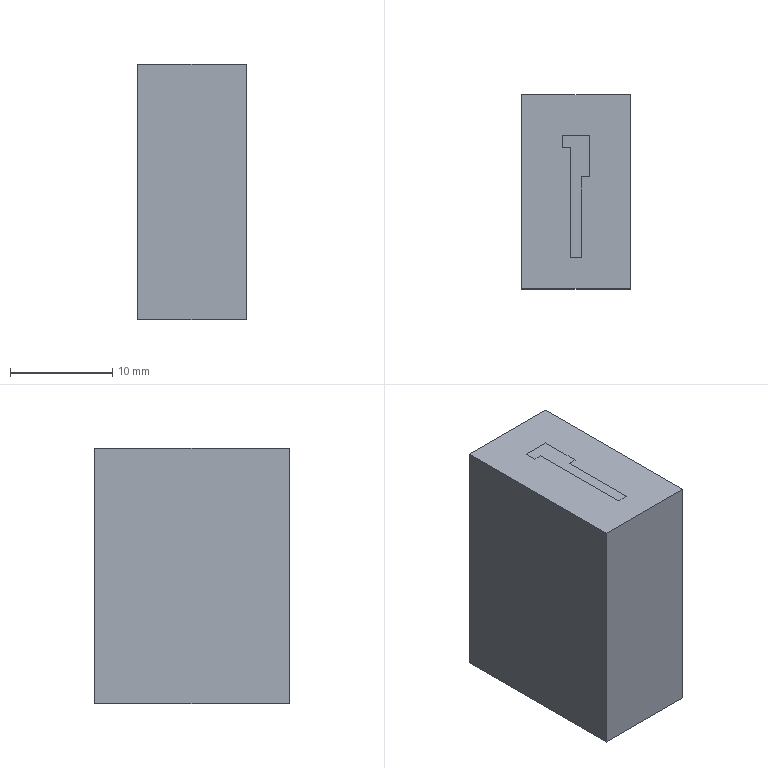Part | NX | features BREP 2 | 2 solids | 29 faces | box 10.58 x 19 x 25 mm | volume 8888 mm3 | plane 29
STEP:
#1=CARTESIAN_POINT('',(-5.29,-9.052,-25.6));
#2=VERTEX_POINT('',#1);
#3=CARTESIAN_POINT('',(-5.29,9.948,-25.6));
#4=VERTEX_POINT('',#3);
#5=CARTESIAN_POINT('',(-5.29,-9.052,-25.6));
#6=DIRECTION('',(0.,1.,0.));
#7=VECTOR('',#6,1000.);
#8=LINE('',#5,#7);
#9=EDGE_CURVE('',#2,#4,#8,.T.);
#10=ORIENTED_EDGE('',*,*,#9,.T.);
#11=CARTESIAN_POINT('',(5.29,9.948,-25.6));
#12=VERTEX_POINT('',#11);
#13=CARTESIAN_POINT('',(-5.29,9.948,-25.6));
#14=DIRECTION('',(1.,0.,0.));
#15=VECTOR('',#14,1000.);
#16=LINE('',#13,#15);
#17=EDGE_CURVE('',#4,#12,#16,.T.);
#18=ORIENTED_EDGE('',*,*,#17,.T.);
#19=CARTESIAN_POINT('',(5.29,-9.052,-25.6));
#20=VERTEX_POINT('',#19);
#21=CARTESIAN_POINT('',(5.29,9.948,-25.6));
#22=DIRECTION('',(0.,-1.,0.));
#23=VECTOR('',#22,1000.);
#24=LINE('',#21,#23);
#25=EDGE_CURVE('',#12,#20,#24,.T.);
#26=ORIENTED_EDGE('',*,*,#25,.T.);
#27=CARTESIAN_POINT('',(5.29,-9.052,-25.6));
#28=DIRECTION('',(-1.,0.,0.));
#29=VECTOR('',#28,1000.);
#30=LINE('',#27,#29);
#31=EDGE_CURVE('',#20,#2,#30,.T.);
#32=ORIENTED_EDGE('',*,*,#31,.T.);
#33=EDGE_LOOP('',(#10,#18,#26,#32));
#34=FACE_BOUND('',#33,.T.);
#35=CARTESIAN_POINT('',(-1.54,3.805,-25.6));
#36=VERTEX_POINT('',#35);
#37=CARTESIAN_POINT('',(-1.54,-6.998,-25.6));
#38=VERTEX_POINT('',#37);
#39=CARTESIAN_POINT('',(-1.54,-2.355,-25.6));
#40=DIRECTION('',(0.,-1.,0.));
#41=VECTOR('',#40,1000.);
#42=LINE('',#39,#41);
#43=EDGE_CURVE('',#36,#38,#42,.T.);
#44=ORIENTED_EDGE('',*,*,#43,.T.);
#45=CARTESIAN_POINT('',(1.54,-6.998,-25.6));
#46=VERTEX_POINT('',#45);
#47=CARTESIAN_POINT('',(-7.04,-6.998,-25.6));
#48=DIRECTION('',(1.,0.,0.));
#49=VECTOR('',#48,1000.);
#50=LINE('',#47,#49);
#51=EDGE_CURVE('',#38,#46,#50,.T.);
#52=ORIENTED_EDGE('',*,*,#51,.T.);
#53=CARTESIAN_POINT('',(1.54,0.9052,-25.6));
#54=VERTEX_POINT('',#53);
#55=CARTESIAN_POINT('',(1.54,-5.255,-25.6));
#56=DIRECTION('',(0.,1.,0.));
#57=VECTOR('',#56,1000.);
#58=LINE('',#55,#57);
#59=EDGE_CURVE('',#46,#54,#58,.T.);
#60=ORIENTED_EDGE('',*,*,#59,.T.);
#61=CARTESIAN_POINT('',(2.34,0.9052,-25.6));
#62=VERTEX_POINT('',#61);
#63=CARTESIAN_POINT('',(1.29,0.9052,-25.6));
#64=DIRECTION('',(1.,0.,0.));
#65=VECTOR('',#64,1000.);
#66=LINE('',#63,#65);
#67=EDGE_CURVE('',#54,#62,#66,.T.);
#68=ORIENTED_EDGE('',*,*,#67,.T.);
#69=CARTESIAN_POINT('',(2.34,6.998,-25.6));
#70=VERTEX_POINT('',#69);
#71=CARTESIAN_POINT('',(2.34,5.948,-25.6));
#72=DIRECTION('',(0.,1.,0.));
#73=VECTOR('',#72,1000.);
#74=LINE('',#71,#73);
#75=EDGE_CURVE('',#62,#70,#74,.T.);
#76=ORIENTED_EDGE('',*,*,#75,.T.);
#77=CARTESIAN_POINT('',(-2.34,6.998,-25.6));
#78=VERTEX_POINT('',#77);
#79=CARTESIAN_POINT('',(-7.04,6.998,-25.6));
#80=DIRECTION('',(-1.,0.,0.));
#81=VECTOR('',#80,1000.);
#82=LINE('',#79,#81);
#83=EDGE_CURVE('',#70,#78,#82,.T.);
#84=ORIENTED_EDGE('',*,*,#83,.T.);
#85=CARTESIAN_POINT('',(-2.34,3.805,-25.6));
#86=VERTEX_POINT('',#85);
#87=CARTESIAN_POINT('',(-2.34,4.855,-25.6));
#88=DIRECTION('',(0.,-1.,0.));
#89=VECTOR('',#88,1000.);
#90=LINE('',#87,#89);
#91=EDGE_CURVE('',#78,#86,#90,.T.);
#92=ORIENTED_EDGE('',*,*,#91,.T.);
#93=CARTESIAN_POINT('',(-0.4899,3.805,-25.6));
#94=DIRECTION('',(1.,0.,0.));
#95=VECTOR('',#94,1000.);
#96=LINE('',#93,#95);
#97=EDGE_CURVE('',#86,#36,#96,.T.);
#98=ORIENTED_EDGE('',*,*,#97,.T.);
#99=EDGE_LOOP('',(#44,#52,#60,#68,#76,#84,#92,#98));
#100=FACE_BOUND('',#99,.T.);
#101=CARTESIAN_POINT('',(0.,0.,-25.6));
#102=DIRECTION('',(0.,0.,-1.));
#103=DIRECTION('',(1.,0.,0.));
#104=AXIS2_PLACEMENT_3D('',#101,#102,#103);
#105=PLANE('',#104);
#106=ADVANCED_FACE('',(#34,#100),#105,.T.);
#107=CARTESIAN_POINT('',(-5.29,-9.052,-0.6));
#108=VERTEX_POINT('',#107);
#109=CARTESIAN_POINT('',(-5.29,9.948,-0.6));
#110=VERTEX_POINT('',#109);
#111=CARTESIAN_POINT('',(-5.29,-9.052,-0.6));
#112=DIRECTION('',(0.,1.,0.));
#113=VECTOR('',#112,1000.);
#114=LINE('',#111,#113);
#115=EDGE_CURVE('',#108,#110,#114,.T.);
#116=ORIENTED_EDGE('',*,*,#115,.F.);
#117=CARTESIAN_POINT('',(5.29,-9.052,-0.6));
#118=VERTEX_POINT('',#117);
#119=CARTESIAN_POINT('',(5.29,-9.052,-0.6));
#120=DIRECTION('',(-1.,0.,0.));
#121=VECTOR('',#120,1000.);
#122=LINE('',#119,#121);
#123=EDGE_CURVE('',#118,#108,#122,.T.);
#124=ORIENTED_EDGE('',*,*,#123,.F.);
#125=CARTESIAN_POINT('',(5.29,9.948,-0.6));
#126=VERTEX_POINT('',#125);
#127=CARTESIAN_POINT('',(5.29,9.948,-0.6));
#128=DIRECTION('',(0.,-1.,0.));
#129=VECTOR('',#128,1000.);
#130=LINE('',#127,#129);
#131=EDGE_CURVE('',#126,#118,#130,.T.);
#132=ORIENTED_EDGE('',*,*,#131,.F.);
#133=CARTESIAN_POINT('',(-5.29,9.948,-0.6));
#134=DIRECTION('',(1.,0.,0.));
#135=VECTOR('',#134,1000.);
#136=LINE('',#133,#135);
#137=EDGE_CURVE('',#110,#126,#136,.T.);
#138=ORIENTED_EDGE('',*,*,#137,.F.);
#139=EDGE_LOOP('',(#116,#124,#132,#138));
#140=FACE_BOUND('',#139,.T.);
#141=CARTESIAN_POINT('',(-0.5399,4.805,-0.6));
#142=VERTEX_POINT('',#141);
#143=CARTESIAN_POINT('',(-0.5399,-5.998,-0.6));
#144=VERTEX_POINT('',#143);
#145=CARTESIAN_POINT('',(-0.5399,-2.355,-0.6));
#146=DIRECTION('',(0.,-1.,0.));
#147=VECTOR('',#146,1000.);
#148=LINE('',#145,#147);
#149=EDGE_CURVE('',#142,#144,#148,.T.);
#150=ORIENTED_EDGE('',*,*,#149,.F.);
#151=CARTESIAN_POINT('',(-1.34,4.805,-0.6));
#152=VERTEX_POINT('',#151);
#153=CARTESIAN_POINT('',(-0.4899,4.805,-0.6));
#154=DIRECTION('',(1.,0.,0.));
#155=VECTOR('',#154,1000.);
#156=LINE('',#153,#155);
#157=EDGE_CURVE('',#152,#142,#156,.T.);
#158=ORIENTED_EDGE('',*,*,#157,.F.);
#159=CARTESIAN_POINT('',(-1.34,5.998,-0.6));
#160=VERTEX_POINT('',#159);
#161=CARTESIAN_POINT('',(-1.34,4.855,-0.6));
#162=DIRECTION('',(0.,-1.,0.));
#163=VECTOR('',#162,1000.);
#164=LINE('',#161,#163);
#165=EDGE_CURVE('',#160,#152,#164,.T.);
#166=ORIENTED_EDGE('',*,*,#165,.F.);
#167=CARTESIAN_POINT('',(1.34,5.998,-0.6));
#168=VERTEX_POINT('',#167);
#169=CARTESIAN_POINT('',(-7.04,5.998,-0.6));
#170=DIRECTION('',(-1.,0.,0.));
#171=VECTOR('',#170,1000.);
#172=LINE('',#169,#171);
#173=EDGE_CURVE('',#168,#160,#172,.T.);
#174=ORIENTED_EDGE('',*,*,#173,.F.);
#175=CARTESIAN_POINT('',(1.34,1.905,-0.6));
#176=VERTEX_POINT('',#175);
#177=CARTESIAN_POINT('',(1.34,5.948,-0.6));
#178=DIRECTION('',(0.,1.,0.));
#179=VECTOR('',#178,1000.);
#180=LINE('',#177,#179);
#181=EDGE_CURVE('',#176,#168,#180,.T.);
#182=ORIENTED_EDGE('',*,*,#181,.F.);
#183=CARTESIAN_POINT('',(0.5399,1.905,-0.6));
#184=VERTEX_POINT('',#183);
#185=CARTESIAN_POINT('',(1.29,1.905,-0.6));
#186=DIRECTION('',(1.,0.,0.));
#187=VECTOR('',#186,1000.);
#188=LINE('',#185,#187);
#189=EDGE_CURVE('',#184,#176,#188,.T.);
#190=ORIENTED_EDGE('',*,*,#189,.F.);
#191=CARTESIAN_POINT('',(0.5399,-5.998,-0.6));
#192=VERTEX_POINT('',#191);
#193=CARTESIAN_POINT('',(0.5399,-5.255,-0.6));
#194=DIRECTION('',(0.,1.,0.));
#195=VECTOR('',#194,1000.);
#196=LINE('',#193,#195);
#197=EDGE_CURVE('',#192,#184,#196,.T.);
#198=ORIENTED_EDGE('',*,*,#197,.F.);
#199=CARTESIAN_POINT('',(-7.04,-5.998,-0.6));
#200=DIRECTION('',(1.,0.,0.));
#201=VECTOR('',#200,1000.);
#202=LINE('',#199,#201);
#203=EDGE_CURVE('',#144,#192,#202,.T.);
#204=ORIENTED_EDGE('',*,*,#203,.F.);
#205=EDGE_LOOP('',(#150,#158,#166,#174,#182,#190,#198,#204));
#206=FACE_BOUND('',#205,.T.);
#207=CARTESIAN_POINT('',(0.,0.,-0.6));
#208=DIRECTION('',(0.,0.,-1.));
#209=DIRECTION('',(1.,0.,0.));
#210=AXIS2_PLACEMENT_3D('',#207,#208,#209);
#211=PLANE('',#210);
#212=ADVANCED_FACE('',(#140,#206),#211,.F.);
#213=ORIENTED_EDGE('',*,*,#115,.T.);
#214=CARTESIAN_POINT('',(-5.29,9.948,-25.6));
#215=DIRECTION('',(0.,0.,1.));
#216=VECTOR('',#215,1000.);
#217=LINE('',#214,#216);
#218=EDGE_CURVE('',#4,#110,#217,.T.);
#219=ORIENTED_EDGE('',*,*,#218,.F.);
#220=ORIENTED_EDGE('',*,*,#9,.F.);
#221=CARTESIAN_POINT('',(-5.29,-9.052,-25.6));
#222=DIRECTION('',(0.,0.,1.));
#223=VECTOR('',#222,1000.);
#224=LINE('',#221,#223);
#225=EDGE_CURVE('',#2,#108,#224,.T.);
#226=ORIENTED_EDGE('',*,*,#225,.T.);
#227=EDGE_LOOP('',(#213,#219,#220,#226));
#228=FACE_BOUND('',#227,.T.);
#229=CARTESIAN_POINT('',(-5.29,-9.052,-25.6));
#230=DIRECTION('',(1.,0.,0.));
#231=DIRECTION('',(0.,-1.,0.));
#232=AXIS2_PLACEMENT_3D('',#229,#230,#231);
#233=PLANE('',#232);
#234=ADVANCED_FACE('',(#228),#233,.F.);
#235=ORIENTED_EDGE('',*,*,#137,.T.);
#236=CARTESIAN_POINT('',(5.29,9.948,-25.6));
#237=DIRECTION('',(0.,0.,1.));
#238=VECTOR('',#237,1000.);
#239=LINE('',#236,#238);
#240=EDGE_CURVE('',#12,#126,#239,.T.);
#241=ORIENTED_EDGE('',*,*,#240,.F.);
#242=ORIENTED_EDGE('',*,*,#17,.F.);
#243=ORIENTED_EDGE('',*,*,#218,.T.);
#244=EDGE_LOOP('',(#235,#241,#242,#243));
#245=FACE_BOUND('',#244,.T.);
#246=CARTESIAN_POINT('',(-5.29,9.948,-25.6));
#247=DIRECTION('',(0.,-1.,0.));
#248=DIRECTION('',(0.,0.,1.));
#249=AXIS2_PLACEMENT_3D('',#246,#247,#248);
#250=PLANE('',#249);
#251=ADVANCED_FACE('',(#245),#250,.F.);
#252=ORIENTED_EDGE('',*,*,#131,.T.);
#253=CARTESIAN_POINT('',(5.29,-9.052,-25.6));
#254=DIRECTION('',(0.,0.,1.));
#255=VECTOR('',#254,1000.);
#256=LINE('',#253,#255);
#257=EDGE_CURVE('',#20,#118,#256,.T.);
#258=ORIENTED_EDGE('',*,*,#257,.F.);
#259=ORIENTED_EDGE('',*,*,#25,.F.);
#260=ORIENTED_EDGE('',*,*,#240,.T.);
#261=EDGE_LOOP('',(#252,#258,#259,#260));
#262=FACE_BOUND('',#261,.T.);
#263=CARTESIAN_POINT('',(5.29,9.948,-25.6));
#264=DIRECTION('',(-1.,0.,0.));
#265=DIRECTION('',(0.,1.,0.));
#266=AXIS2_PLACEMENT_3D('',#263,#264,#265);
#267=PLANE('',#266);
#268=ADVANCED_FACE('',(#262),#267,.F.);
#269=ORIENTED_EDGE('',*,*,#123,.T.);
#270=ORIENTED_EDGE('',*,*,#225,.F.);
#271=ORIENTED_EDGE('',*,*,#31,.F.);
#272=ORIENTED_EDGE('',*,*,#257,.T.);
#273=EDGE_LOOP('',(#269,#270,#271,#272));
#274=FACE_BOUND('',#273,.T.);
#275=CARTESIAN_POINT('',(5.29,-9.052,-25.6));
#276=DIRECTION('',(0.,1.,0.));
#277=DIRECTION('',(0.,0.,-1.));
#278=AXIS2_PLACEMENT_3D('',#275,#276,#277);
#279=PLANE('',#278);
#280=ADVANCED_FACE('',(#274),#279,.F.);
#281=CARTESIAN_POINT('',(-0.5399,4.805,-3.6));
#282=VERTEX_POINT('',#281);
#283=CARTESIAN_POINT('',(-0.5399,4.805,0.));
#284=DIRECTION('',(0.,0.,-1.));
#285=VECTOR('',#284,1000.);
#286=LINE('',#283,#285);
#287=EDGE_CURVE('',#142,#282,#286,.T.);
#288=ORIENTED_EDGE('',*,*,#287,.T.);
#289=CARTESIAN_POINT('',(-1.34,4.805,-3.6));
#290=VERTEX_POINT('',#289);
#291=CARTESIAN_POINT('',(-0.4899,4.805,-3.6));
#292=DIRECTION('',(-1.,0.,0.));
#293=VECTOR('',#292,1000.);
#294=LINE('',#291,#293);
#295=EDGE_CURVE('',#282,#290,#294,.T.);
#296=ORIENTED_EDGE('',*,*,#295,.T.);
#297=CARTESIAN_POINT('',(-1.34,4.805,0.));
#298=DIRECTION('',(0.,0.,-1.));
#299=VECTOR('',#298,1000.);
#300=LINE('',#297,#299);
#301=EDGE_CURVE('',#152,#290,#300,.T.);
#302=ORIENTED_EDGE('',*,*,#301,.F.);
#303=ORIENTED_EDGE('',*,*,#157,.T.);
#304=EDGE_LOOP('',(#288,#296,#302,#303));
#305=FACE_BOUND('',#304,.T.);
#306=CARTESIAN_POINT('',(-0.4899,4.805,0.));
#307=DIRECTION('',(0.,1.,0.));
#308=DIRECTION('',(1.,0.,0.));
#309=AXIS2_PLACEMENT_3D('',#306,#307,#308);
#310=PLANE('',#309);
#311=ADVANCED_FACE('',(#305),#310,.T.);
#312=ORIENTED_EDGE('',*,*,#301,.T.);
#313=CARTESIAN_POINT('',(-1.34,5.998,-3.6));
#314=VERTEX_POINT('',#313);
#315=CARTESIAN_POINT('',(-1.34,4.855,-3.6));
#316=DIRECTION('',(0.,1.,0.));
#317=VECTOR('',#316,1000.);
#318=LINE('',#315,#317);
#319=EDGE_CURVE('',#290,#314,#318,.T.);
#320=ORIENTED_EDGE('',*,*,#319,.T.);
#321=CARTESIAN_POINT('',(-1.34,5.998,0.));
#322=DIRECTION('',(0.,0.,-1.));
#323=VECTOR('',#322,1000.);
#324=LINE('',#321,#323);
#325=EDGE_CURVE('',#160,#314,#324,.T.);
#326=ORIENTED_EDGE('',*,*,#325,.F.);
#327=ORIENTED_EDGE('',*,*,#165,.T.);
#328=EDGE_LOOP('',(#312,#320,#326,#327));
#329=FACE_BOUND('',#328,.T.);
#330=CARTESIAN_POINT('',(-1.34,4.855,0.));
#331=DIRECTION('',(1.,0.,0.));
#332=DIRECTION('',(0.,-1.,0.));
#333=AXIS2_PLACEMENT_3D('',#330,#331,#332);
#334=PLANE('',#333);
#335=ADVANCED_FACE('',(#329),#334,.T.);
#336=ORIENTED_EDGE('',*,*,#325,.T.);
#337=CARTESIAN_POINT('',(1.34,5.998,-3.6));
#338=VERTEX_POINT('',#337);
#339=CARTESIAN_POINT('',(-7.04,5.998,-3.6));
#340=DIRECTION('',(1.,0.,0.));
#341=VECTOR('',#340,1000.);
#342=LINE('',#339,#341);
#343=EDGE_CURVE('',#314,#338,#342,.T.);
#344=ORIENTED_EDGE('',*,*,#343,.T.);
#345=CARTESIAN_POINT('',(1.34,5.998,0.));
#346=DIRECTION('',(0.,0.,-1.));
#347=VECTOR('',#346,1000.);
#348=LINE('',#345,#347);
#349=EDGE_CURVE('',#168,#338,#348,.T.);
#350=ORIENTED_EDGE('',*,*,#349,.F.);
#351=ORIENTED_EDGE('',*,*,#173,.T.);
#352=EDGE_LOOP('',(#336,#344,#350,#351));
#353=FACE_BOUND('',#352,.T.);
#354=CARTESIAN_POINT('',(-7.04,5.998,0.));
#355=DIRECTION('',(0.,1.,0.));
#356=DIRECTION('',(1.,0.,0.));
#357=AXIS2_PLACEMENT_3D('',#354,#355,#356);
#358=PLANE('',#357);
#359=ADVANCED_FACE('',(#353),#358,.F.);
#360=ORIENTED_EDGE('',*,*,#349,.T.);
#361=CARTESIAN_POINT('',(1.34,1.905,-3.6));
#362=VERTEX_POINT('',#361);
#363=CARTESIAN_POINT('',(1.34,5.948,-3.6));
#364=DIRECTION('',(0.,-1.,0.));
#365=VECTOR('',#364,1000.);
#366=LINE('',#363,#365);
#367=EDGE_CURVE('',#338,#362,#366,.T.);
#368=ORIENTED_EDGE('',*,*,#367,.T.);
#369=CARTESIAN_POINT('',(1.34,1.905,0.));
#370=DIRECTION('',(0.,0.,-1.));
#371=VECTOR('',#370,1000.);
#372=LINE('',#369,#371);
#373=EDGE_CURVE('',#176,#362,#372,.T.);
#374=ORIENTED_EDGE('',*,*,#373,.F.);
#375=ORIENTED_EDGE('',*,*,#181,.T.);
#376=EDGE_LOOP('',(#360,#368,#374,#375));
#377=FACE_BOUND('',#376,.T.);
#378=CARTESIAN_POINT('',(1.34,5.948,0.));
#379=DIRECTION('',(-1.,0.,0.));
#380=DIRECTION('',(0.,1.,0.));
#381=AXIS2_PLACEMENT_3D('',#378,#379,#380);
#382=PLANE('',#381);
#383=ADVANCED_FACE('',(#377),#382,.T.);
#384=ORIENTED_EDGE('',*,*,#373,.T.);
#385=CARTESIAN_POINT('',(0.5399,1.905,-3.6));
#386=VERTEX_POINT('',#385);
#387=CARTESIAN_POINT('',(1.29,1.905,-3.6));
#388=DIRECTION('',(-1.,0.,0.));
#389=VECTOR('',#388,1000.);
#390=LINE('',#387,#389);
#391=EDGE_CURVE('',#362,#386,#390,.T.);
#392=ORIENTED_EDGE('',*,*,#391,.T.);
#393=CARTESIAN_POINT('',(0.5399,1.905,0.));
#394=DIRECTION('',(0.,0.,-1.));
#395=VECTOR('',#394,1000.);
#396=LINE('',#393,#395);
#397=EDGE_CURVE('',#184,#386,#396,.T.);
#398=ORIENTED_EDGE('',*,*,#397,.F.);
#399=ORIENTED_EDGE('',*,*,#189,.T.);
#400=EDGE_LOOP('',(#384,#392,#398,#399));
#401=FACE_BOUND('',#400,.T.);
#402=CARTESIAN_POINT('',(1.29,1.905,0.));
#403=DIRECTION('',(0.,1.,0.));
#404=DIRECTION('',(1.,0.,0.));
#405=AXIS2_PLACEMENT_3D('',#402,#403,#404);
#406=PLANE('',#405);
#407=ADVANCED_FACE('',(#401),#406,.T.);
#408=CARTESIAN_POINT('',(0.5399,-5.998,-3.6));
#409=VERTEX_POINT('',#408);
#410=CARTESIAN_POINT('',(0.5399,-5.998,0.));
#411=DIRECTION('',(0.,0.,-1.));
#412=VECTOR('',#411,1000.);
#413=LINE('',#410,#412);
#414=EDGE_CURVE('',#192,#409,#413,.T.);
#415=ORIENTED_EDGE('',*,*,#414,.F.);
#416=ORIENTED_EDGE('',*,*,#197,.T.);
#417=ORIENTED_EDGE('',*,*,#397,.T.);
#418=CARTESIAN_POINT('',(0.5399,-5.255,-3.6));
#419=DIRECTION('',(0.,-1.,0.));
#420=VECTOR('',#419,1000.);
#421=LINE('',#418,#420);
#422=EDGE_CURVE('',#386,#409,#421,.T.);
#423=ORIENTED_EDGE('',*,*,#422,.T.);
#424=EDGE_LOOP('',(#415,#416,#417,#423));
#425=FACE_BOUND('',#424,.T.);
#426=CARTESIAN_POINT('',(0.5399,-5.255,0.));
#427=DIRECTION('',(-1.,0.,0.));
#428=DIRECTION('',(0.,1.,0.));
#429=AXIS2_PLACEMENT_3D('',#426,#427,#428);
#430=PLANE('',#429);
#431=ADVANCED_FACE('',(#425),#430,.T.);
#432=ORIENTED_EDGE('',*,*,#414,.T.);
#433=CARTESIAN_POINT('',(-0.5399,-5.998,-3.6));
#434=VERTEX_POINT('',#433);
#435=CARTESIAN_POINT('',(-7.04,-5.998,-3.6));
#436=DIRECTION('',(-1.,0.,0.));
#437=VECTOR('',#436,1000.);
#438=LINE('',#435,#437);
#439=EDGE_CURVE('',#409,#434,#438,.T.);
#440=ORIENTED_EDGE('',*,*,#439,.T.);
#441=CARTESIAN_POINT('',(-0.5399,-5.998,0.));
#442=DIRECTION('',(0.,0.,-1.));
#443=VECTOR('',#442,1000.);
#444=LINE('',#441,#443);
#445=EDGE_CURVE('',#144,#434,#444,.T.);
#446=ORIENTED_EDGE('',*,*,#445,.F.);
#447=ORIENTED_EDGE('',*,*,#203,.T.);
#448=EDGE_LOOP('',(#432,#440,#446,#447));
#449=FACE_BOUND('',#448,.T.);
#450=CARTESIAN_POINT('',(-7.04,-5.998,0.));
#451=DIRECTION('',(0.,-1.,0.));
#452=DIRECTION('',(-1.,0.,0.));
#453=AXIS2_PLACEMENT_3D('',#450,#451,#452);
#454=PLANE('',#453);
#455=ADVANCED_FACE('',(#449),#454,.F.);
#456=CARTESIAN_POINT('',(-0.5399,-2.355,-3.6));
#457=DIRECTION('',(0.,1.,0.));
#458=VECTOR('',#457,1000.);
#459=LINE('',#456,#458);
#460=EDGE_CURVE('',#434,#282,#459,.T.);
#461=ORIENTED_EDGE('',*,*,#460,.T.);
#462=ORIENTED_EDGE('',*,*,#287,.F.);
#463=ORIENTED_EDGE('',*,*,#149,.T.);
#464=ORIENTED_EDGE('',*,*,#445,.T.);
#465=EDGE_LOOP('',(#461,#462,#463,#464));
#466=FACE_BOUND('',#465,.T.);
#467=CARTESIAN_POINT('',(-0.5399,-2.355,0.));
#468=DIRECTION('',(1.,0.,0.));
#469=DIRECTION('',(0.,-1.,0.));
#470=AXIS2_PLACEMENT_3D('',#467,#468,#469);
#471=PLANE('',#470);
#472=ADVANCED_FACE('',(#466),#471,.T.);
#473=CARTESIAN_POINT('',(1.54,-6.998,-3.6));
#474=VERTEX_POINT('',#473);
#475=CARTESIAN_POINT('',(-1.54,-6.998,-3.6));
#476=VERTEX_POINT('',#475);
#477=CARTESIAN_POINT('',(-7.04,-6.998,-3.6));
#478=DIRECTION('',(-1.,0.,0.));
#479=VECTOR('',#478,1000.);
#480=LINE('',#477,#479);
#481=EDGE_CURVE('',#474,#476,#480,.T.);
#482=ORIENTED_EDGE('',*,*,#481,.T.);
#483=CARTESIAN_POINT('',(-1.54,3.805,-3.6));
#484=VERTEX_POINT('',#483);
#485=CARTESIAN_POINT('',(-1.54,-2.355,-3.6));
#486=DIRECTION('',(0.,1.,0.));
#487=VECTOR('',#486,1000.);
#488=LINE('',#485,#487);
#489=EDGE_CURVE('',#476,#484,#488,.T.);
#490=ORIENTED_EDGE('',*,*,#489,.T.);
#491=CARTESIAN_POINT('',(-2.34,3.805,-3.6));
#492=VERTEX_POINT('',#491);
#493=CARTESIAN_POINT('',(-0.4899,3.805,-3.6));
#494=DIRECTION('',(-1.,0.,0.));
#495=VECTOR('',#494,1000.);
#496=LINE('',#493,#495);
#497=EDGE_CURVE('',#484,#492,#496,.T.);
#498=ORIENTED_EDGE('',*,*,#497,.T.);
#499=CARTESIAN_POINT('',(-2.34,6.998,-3.6));
#500=VERTEX_POINT('',#499);
#501=CARTESIAN_POINT('',(-2.34,4.855,-3.6));
#502=DIRECTION('',(0.,1.,0.));
#503=VECTOR('',#502,1000.);
#504=LINE('',#501,#503);
#505=EDGE_CURVE('',#492,#500,#504,.T.);
#506=ORIENTED_EDGE('',*,*,#505,.T.);
#507=CARTESIAN_POINT('',(2.34,6.998,-3.6));
#508=VERTEX_POINT('',#507);
#509=CARTESIAN_POINT('',(-7.04,6.998,-3.6));
#510=DIRECTION('',(1.,0.,0.));
#511=VECTOR('',#510,1000.);
#512=LINE('',#509,#511);
#513=EDGE_CURVE('',#500,#508,#512,.T.);
#514=ORIENTED_EDGE('',*,*,#513,.T.);
#515=CARTESIAN_POINT('',(2.34,0.9052,-3.6));
#516=VERTEX_POINT('',#515);
#517=CARTESIAN_POINT('',(2.34,5.948,-3.6));
#518=DIRECTION('',(0.,-1.,0.));
#519=VECTOR('',#518,1000.);
#520=LINE('',#517,#519);
#521=EDGE_CURVE('',#508,#516,#520,.T.);
#522=ORIENTED_EDGE('',*,*,#521,.T.);
#523=CARTESIAN_POINT('',(1.54,0.9052,-3.6));
#524=VERTEX_POINT('',#523);
#525=CARTESIAN_POINT('',(1.29,0.9052,-3.6));
#526=DIRECTION('',(-1.,0.,0.));
#527=VECTOR('',#526,1000.);
#528=LINE('',#525,#527);
#529=EDGE_CURVE('',#516,#524,#528,.T.);
#530=ORIENTED_EDGE('',*,*,#529,.T.);
#531=CARTESIAN_POINT('',(1.54,-5.255,-3.6));
#532=DIRECTION('',(0.,-1.,0.));
#533=VECTOR('',#532,1000.);
#534=LINE('',#531,#533);
#535=EDGE_CURVE('',#524,#474,#534,.T.);
#536=ORIENTED_EDGE('',*,*,#535,.T.);
#537=EDGE_LOOP('',(#482,#490,#498,#506,#514,#522,#530,#536));
#538=FACE_BOUND('',#537,.T.);
#539=ORIENTED_EDGE('',*,*,#422,.F.);
#540=ORIENTED_EDGE('',*,*,#391,.F.);
#541=ORIENTED_EDGE('',*,*,#367,.F.);
#542=ORIENTED_EDGE('',*,*,#343,.F.);
#543=ORIENTED_EDGE('',*,*,#319,.F.);
#544=ORIENTED_EDGE('',*,*,#295,.F.);
#545=ORIENTED_EDGE('',*,*,#460,.F.);
#546=ORIENTED_EDGE('',*,*,#439,.F.);
#547=EDGE_LOOP('',(#539,#540,#541,#542,#543,#544,#545,#546));
#548=FACE_BOUND('',#547,.T.);
#549=CARTESIAN_POINT('',(-7.04,-19.654,-3.6));
#550=DIRECTION('',(0.,0.,1.));
#551=DIRECTION('',(-1.,0.,0.));
#552=AXIS2_PLACEMENT_3D('',#549,#550,#551);
#553=PLANE('',#552);
#554=ADVANCED_FACE('',(#538,#548),#553,.F.);
#555=CARTESIAN_POINT('',(-1.54,3.805,-3.6));
#556=DIRECTION('',(0.,0.,-1.));
#557=VECTOR('',#556,1000.);
#558=LINE('',#555,#557);
#559=EDGE_CURVE('',#484,#36,#558,.T.);
#560=ORIENTED_EDGE('',*,*,#559,.T.);
#561=ORIENTED_EDGE('',*,*,#97,.F.);
#562=CARTESIAN_POINT('',(-2.34,3.805,-3.6));
#563=DIRECTION('',(0.,0.,-1.));
#564=VECTOR('',#563,1000.);
#565=LINE('',#562,#564);
#566=EDGE_CURVE('',#492,#86,#565,.T.);
#567=ORIENTED_EDGE('',*,*,#566,.F.);
#568=ORIENTED_EDGE('',*,*,#497,.F.);
#569=EDGE_LOOP('',(#560,#561,#567,#568));
#570=FACE_BOUND('',#569,.T.);
#571=CARTESIAN_POINT('',(-0.4899,3.805,-3.6));
#572=DIRECTION('',(0.,-1.,0.));
#573=DIRECTION('',(-1.,0.,0.));
#574=AXIS2_PLACEMENT_3D('',#571,#572,#573);
#575=PLANE('',#574);
#576=ADVANCED_FACE('',(#570),#575,.F.);
#577=ORIENTED_EDGE('',*,*,#566,.T.);
#578=ORIENTED_EDGE('',*,*,#91,.F.);
#579=CARTESIAN_POINT('',(-2.34,6.998,-3.6));
#580=DIRECTION('',(0.,0.,-1.));
#581=VECTOR('',#580,1000.);
#582=LINE('',#579,#581);
#583=EDGE_CURVE('',#500,#78,#582,.T.);
#584=ORIENTED_EDGE('',*,*,#583,.F.);
#585=ORIENTED_EDGE('',*,*,#505,.F.);
#586=EDGE_LOOP('',(#577,#578,#584,#585));
#587=FACE_BOUND('',#586,.T.);
#588=CARTESIAN_POINT('',(-2.34,4.855,-3.6));
#589=DIRECTION('',(-1.,0.,0.));
#590=DIRECTION('',(0.,1.,0.));
#591=AXIS2_PLACEMENT_3D('',#588,#589,#590);
#592=PLANE('',#591);
#593=ADVANCED_FACE('',(#587),#592,.F.);
#594=ORIENTED_EDGE('',*,*,#583,.T.);
#595=ORIENTED_EDGE('',*,*,#83,.F.);
#596=CARTESIAN_POINT('',(2.34,6.998,-3.6));
#597=DIRECTION('',(0.,0.,-1.));
#598=VECTOR('',#597,1000.);
#599=LINE('',#596,#598);
#600=EDGE_CURVE('',#508,#70,#599,.T.);
#601=ORIENTED_EDGE('',*,*,#600,.F.);
#602=ORIENTED_EDGE('',*,*,#513,.F.);
#603=EDGE_LOOP('',(#594,#595,#601,#602));
#604=FACE_BOUND('',#603,.T.);
#605=CARTESIAN_POINT('',(-7.04,6.998,-3.6));
#606=DIRECTION('',(0.,-1.,0.));
#607=DIRECTION('',(-1.,0.,0.));
#608=AXIS2_PLACEMENT_3D('',#605,#606,#607);
#609=PLANE('',#608);
#610=ADVANCED_FACE('',(#604),#609,.T.);
#611=ORIENTED_EDGE('',*,*,#600,.T.);
#612=ORIENTED_EDGE('',*,*,#75,.F.);
#613=CARTESIAN_POINT('',(2.34,0.9052,-3.6));
#614=DIRECTION('',(0.,0.,-1.));
#615=VECTOR('',#614,1000.);
#616=LINE('',#613,#615);
#617=EDGE_CURVE('',#516,#62,#616,.T.);
#618=ORIENTED_EDGE('',*,*,#617,.F.);
#619=ORIENTED_EDGE('',*,*,#521,.F.);
#620=EDGE_LOOP('',(#611,#612,#618,#619));
#621=FACE_BOUND('',#620,.T.);
#622=CARTESIAN_POINT('',(2.34,5.948,-3.6));
#623=DIRECTION('',(1.,0.,0.));
#624=DIRECTION('',(0.,-1.,0.));
#625=AXIS2_PLACEMENT_3D('',#622,#623,#624);
#626=PLANE('',#625);
#627=ADVANCED_FACE('',(#621),#626,.F.);
#628=ORIENTED_EDGE('',*,*,#617,.T.);
#629=ORIENTED_EDGE('',*,*,#67,.F.);
#630=CARTESIAN_POINT('',(1.54,0.9052,-3.6));
#631=DIRECTION('',(0.,0.,-1.));
#632=VECTOR('',#631,1000.);
#633=LINE('',#630,#632);
#634=EDGE_CURVE('',#524,#54,#633,.T.);
#635=ORIENTED_EDGE('',*,*,#634,.F.);
#636=ORIENTED_EDGE('',*,*,#529,.F.);
#637=EDGE_LOOP('',(#628,#629,#635,#636));
#638=FACE_BOUND('',#637,.T.);
#639=CARTESIAN_POINT('',(1.29,0.9052,-3.6));
#640=DIRECTION('',(0.,-1.,0.));
#641=DIRECTION('',(-1.,0.,0.));
#642=AXIS2_PLACEMENT_3D('',#639,#640,#641);
#643=PLANE('',#642);
#644=ADVANCED_FACE('',(#638),#643,.F.);
#645=ORIENTED_EDGE('',*,*,#634,.T.);
#646=ORIENTED_EDGE('',*,*,#59,.F.);
#647=CARTESIAN_POINT('',(1.54,-6.998,-3.6));
#648=DIRECTION('',(0.,0.,-1.));
#649=VECTOR('',#648,1000.);
#650=LINE('',#647,#649);
#651=EDGE_CURVE('',#474,#46,#650,.T.);
#652=ORIENTED_EDGE('',*,*,#651,.F.);
#653=ORIENTED_EDGE('',*,*,#535,.F.);
#654=EDGE_LOOP('',(#645,#646,#652,#653));
#655=FACE_BOUND('',#654,.T.);
#656=CARTESIAN_POINT('',(1.54,-5.255,-3.6));
#657=DIRECTION('',(1.,0.,0.));
#658=DIRECTION('',(0.,-1.,0.));
#659=AXIS2_PLACEMENT_3D('',#656,#657,#658);
#660=PLANE('',#659);
#661=ADVANCED_FACE('',(#655),#660,.F.);
#662=ORIENTED_EDGE('',*,*,#651,.T.);
#663=ORIENTED_EDGE('',*,*,#51,.F.);
#664=CARTESIAN_POINT('',(-1.54,-6.998,-3.6));
#665=DIRECTION('',(0.,0.,-1.));
#666=VECTOR('',#665,1000.);
#667=LINE('',#664,#666);
#668=EDGE_CURVE('',#476,#38,#667,.T.);
#669=ORIENTED_EDGE('',*,*,#668,.F.);
#670=ORIENTED_EDGE('',*,*,#481,.F.);
#671=EDGE_LOOP('',(#662,#663,#669,#670));
#672=FACE_BOUND('',#671,.T.);
#673=CARTESIAN_POINT('',(-7.04,-6.998,-3.6));
#674=DIRECTION('',(0.,1.,0.));
#675=DIRECTION('',(1.,0.,0.));
#676=AXIS2_PLACEMENT_3D('',#673,#674,#675);
#677=PLANE('',#676);
#678=ADVANCED_FACE('',(#672),#677,.T.);
#679=ORIENTED_EDGE('',*,*,#43,.F.);
#680=ORIENTED_EDGE('',*,*,#559,.F.);
#681=ORIENTED_EDGE('',*,*,#489,.F.);
#682=ORIENTED_EDGE('',*,*,#668,.T.);
#683=EDGE_LOOP('',(#679,#680,#681,#682));
#684=FACE_BOUND('',#683,.T.);
#685=CARTESIAN_POINT('',(-1.54,-2.355,-3.6));
#686=DIRECTION('',(-1.,0.,0.));
#687=DIRECTION('',(0.,1.,0.));
#688=AXIS2_PLACEMENT_3D('',#685,#686,#687);
#689=PLANE('',#688);
#690=ADVANCED_FACE('',(#684),#689,.F.);
#691=CLOSED_SHELL('',(#106,#212,#234,#251,#268,#280,#311,#335,#359,#383,#407,#431,#455,#472,#554,#576,#593,#610,#627,#644,#661,#678,#690));
#692=MANIFOLD_SOLID_BREP('',#691);
#693=CARTESIAN_POINT('',(-5.29,-9.052,-0.6));
#694=VERTEX_POINT('',#693);
#695=CARTESIAN_POINT('',(-5.29,9.948,-0.6));
#696=VERTEX_POINT('',#695);
#697=CARTESIAN_POINT('',(-5.29,-9.052,-0.6));
#698=DIRECTION('',(0.,1.,0.));
#699=VECTOR('',#698,1000.);
#700=LINE('',#697,#699);
#701=EDGE_CURVE('',#694,#696,#700,.T.);
#702=ORIENTED_EDGE('',*,*,#701,.T.);
#703=CARTESIAN_POINT('',(-5.29,9.948,-25.6));
#704=VERTEX_POINT('',#703);
#705=CARTESIAN_POINT('',(-5.29,9.948,-25.6));
#706=DIRECTION('',(0.,0.,1.));
#707=VECTOR('',#706,1000.);
#708=LINE('',#705,#707);
#709=EDGE_CURVE('',#704,#696,#708,.T.);
#710=ORIENTED_EDGE('',*,*,#709,.F.);
#711=CARTESIAN_POINT('',(-5.29,-9.052,-25.6));
#712=VERTEX_POINT('',#711);
#713=CARTESIAN_POINT('',(-5.29,-9.052,-25.6));
#714=DIRECTION('',(0.,1.,0.));
#715=VECTOR('',#714,1000.);
#716=LINE('',#713,#715);
#717=EDGE_CURVE('',#712,#704,#716,.T.);
#718=ORIENTED_EDGE('',*,*,#717,.F.);
#719=CARTESIAN_POINT('',(-5.29,-9.052,-25.6));
#720=DIRECTION('',(0.,0.,1.));
#721=VECTOR('',#720,1000.);
#722=LINE('',#719,#721);
#723=EDGE_CURVE('',#712,#694,#722,.T.);
#724=ORIENTED_EDGE('',*,*,#723,.T.);
#725=EDGE_LOOP('',(#702,#710,#718,#724));
#726=FACE_BOUND('',#725,.T.);
#727=CARTESIAN_POINT('',(-5.29,-9.052,-25.6));
#728=DIRECTION('',(1.,0.,0.));
#729=DIRECTION('',(0.,-1.,0.));
#730=AXIS2_PLACEMENT_3D('',#727,#728,#729);
#731=PLANE('',#730);
#732=ADVANCED_FACE('',(#726),#731,.F.);
#733=CARTESIAN_POINT('',(5.29,9.948,-0.6));
#734=VERTEX_POINT('',#733);
#735=CARTESIAN_POINT('',(-5.29,9.948,-0.6));
#736=DIRECTION('',(1.,0.,0.));
#737=VECTOR('',#736,1000.);
#738=LINE('',#735,#737);
#739=EDGE_CURVE('',#696,#734,#738,.T.);
#740=ORIENTED_EDGE('',*,*,#739,.T.);
#741=CARTESIAN_POINT('',(5.29,9.948,-25.6));
#742=VERTEX_POINT('',#741);
#743=CARTESIAN_POINT('',(5.29,9.948,-25.6));
#744=DIRECTION('',(0.,0.,1.));
#745=VECTOR('',#744,1000.);
#746=LINE('',#743,#745);
#747=EDGE_CURVE('',#742,#734,#746,.T.);
#748=ORIENTED_EDGE('',*,*,#747,.F.);
#749=CARTESIAN_POINT('',(-5.29,9.948,-25.6));
#750=DIRECTION('',(1.,0.,0.));
#751=VECTOR('',#750,1000.);
#752=LINE('',#749,#751);
#753=EDGE_CURVE('',#704,#742,#752,.T.);
#754=ORIENTED_EDGE('',*,*,#753,.F.);
#755=ORIENTED_EDGE('',*,*,#709,.T.);
#756=EDGE_LOOP('',(#740,#748,#754,#755));
#757=FACE_BOUND('',#756,.T.);
#758=CARTESIAN_POINT('',(-5.29,9.948,-25.6));
#759=DIRECTION('',(0.,-1.,0.));
#760=DIRECTION('',(0.,0.,1.));
#761=AXIS2_PLACEMENT_3D('',#758,#759,#760);
#762=PLANE('',#761);
#763=ADVANCED_FACE('',(#757),#762,.F.);
#764=CARTESIAN_POINT('',(5.29,-9.052,-0.6));
#765=VERTEX_POINT('',#764);
#766=CARTESIAN_POINT('',(5.29,9.948,-0.6));
#767=DIRECTION('',(0.,-1.,0.));
#768=VECTOR('',#767,1000.);
#769=LINE('',#766,#768);
#770=EDGE_CURVE('',#734,#765,#769,.T.);
#771=ORIENTED_EDGE('',*,*,#770,.T.);
#772=CARTESIAN_POINT('',(5.29,-9.052,-25.6));
#773=VERTEX_POINT('',#772);
#774=CARTESIAN_POINT('',(5.29,-9.052,-25.6));
#775=DIRECTION('',(0.,0.,1.));
#776=VECTOR('',#775,1000.);
#777=LINE('',#774,#776);
#778=EDGE_CURVE('',#773,#765,#777,.T.);
#779=ORIENTED_EDGE('',*,*,#778,.F.);
#780=CARTESIAN_POINT('',(5.29,9.948,-25.6));
#781=DIRECTION('',(0.,-1.,0.));
#782=VECTOR('',#781,1000.);
#783=LINE('',#780,#782);
#784=EDGE_CURVE('',#742,#773,#783,.T.);
#785=ORIENTED_EDGE('',*,*,#784,.F.);
#786=ORIENTED_EDGE('',*,*,#747,.T.);
#787=EDGE_LOOP('',(#771,#779,#785,#786));
#788=FACE_BOUND('',#787,.T.);
#789=CARTESIAN_POINT('',(5.29,9.948,-25.6));
#790=DIRECTION('',(-1.,0.,0.));
#791=DIRECTION('',(0.,1.,0.));
#792=AXIS2_PLACEMENT_3D('',#789,#790,#791);
#793=PLANE('',#792);
#794=ADVANCED_FACE('',(#788),#793,.F.);
#795=CARTESIAN_POINT('',(5.29,-9.052,-0.6));
#796=DIRECTION('',(-1.,0.,0.));
#797=VECTOR('',#796,1000.);
#798=LINE('',#795,#797);
#799=EDGE_CURVE('',#765,#694,#798,.T.);
#800=ORIENTED_EDGE('',*,*,#799,.T.);
#801=ORIENTED_EDGE('',*,*,#723,.F.);
#802=CARTESIAN_POINT('',(5.29,-9.052,-25.6));
#803=DIRECTION('',(-1.,0.,0.));
#804=VECTOR('',#803,1000.);
#805=LINE('',#802,#804);
#806=EDGE_CURVE('',#773,#712,#805,.T.);
#807=ORIENTED_EDGE('',*,*,#806,.F.);
#808=ORIENTED_EDGE('',*,*,#778,.T.);
#809=EDGE_LOOP('',(#800,#801,#807,#808));
#810=FACE_BOUND('',#809,.T.);
#811=CARTESIAN_POINT('',(5.29,-9.052,-25.6));
#812=DIRECTION('',(0.,1.,0.));
#813=DIRECTION('',(0.,0.,-1.));
#814=AXIS2_PLACEMENT_3D('',#811,#812,#813);
#815=PLANE('',#814);
#816=ADVANCED_FACE('',(#810),#815,.F.);
#817=ORIENTED_EDGE('',*,*,#717,.T.);
#818=ORIENTED_EDGE('',*,*,#753,.T.);
#819=ORIENTED_EDGE('',*,*,#784,.T.);
#820=ORIENTED_EDGE('',*,*,#806,.T.);
#821=EDGE_LOOP('',(#817,#818,#819,#820));
#822=FACE_BOUND('',#821,.T.);
#823=CARTESIAN_POINT('',(0.,0.,-25.6));
#824=DIRECTION('',(0.,0.,-1.));
#825=DIRECTION('',(1.,0.,0.));
#826=AXIS2_PLACEMENT_3D('',#823,#824,#825);
#827=PLANE('',#826);
#828=ADVANCED_FACE('',(#822),#827,.T.);
#829=ORIENTED_EDGE('',*,*,#701,.F.);
#830=ORIENTED_EDGE('',*,*,#799,.F.);
#831=ORIENTED_EDGE('',*,*,#770,.F.);
#832=ORIENTED_EDGE('',*,*,#739,.F.);
#833=EDGE_LOOP('',(#829,#830,#831,#832));
#834=FACE_BOUND('',#833,.T.);
#835=CARTESIAN_POINT('',(0.,0.,-0.6));
#836=DIRECTION('',(0.,0.,-1.));
#837=DIRECTION('',(1.,0.,0.));
#838=AXIS2_PLACEMENT_3D('',#835,#836,#837);
#839=PLANE('',#838);
#840=ADVANCED_FACE('',(#834),#839,.F.);
#841=CLOSED_SHELL('',(#732,#763,#794,#816,#828,#840));
#842=MANIFOLD_SOLID_BREP('',#841);
#843=(LENGTH_UNIT()NAMED_UNIT(*)SI_UNIT(.MILLI.,.METRE.));
#844=UNCERTAINTY_MEASURE_WITH_UNIT(LENGTH_MEASURE(0.00001),#843,'','');
#845=(NAMED_UNIT(*)PLANE_ANGLE_UNIT()SI_UNIT($,.RADIAN.));
#846=(NAMED_UNIT(*)SI_UNIT($,.STERADIAN.)SOLID_ANGLE_UNIT());
#847=(GEOMETRIC_REPRESENTATION_CONTEXT(3)GLOBAL_UNCERTAINTY_ASSIGNED_CONTEXT((#844))GLOBAL_UNIT_ASSIGNED_CONTEXT((#843,#845,#846))REPRESENTATION_CONTEXT('',''));
#848=ADVANCED_BREP_SHAPE_REPRESENTATION('',(#692,#842),#847);